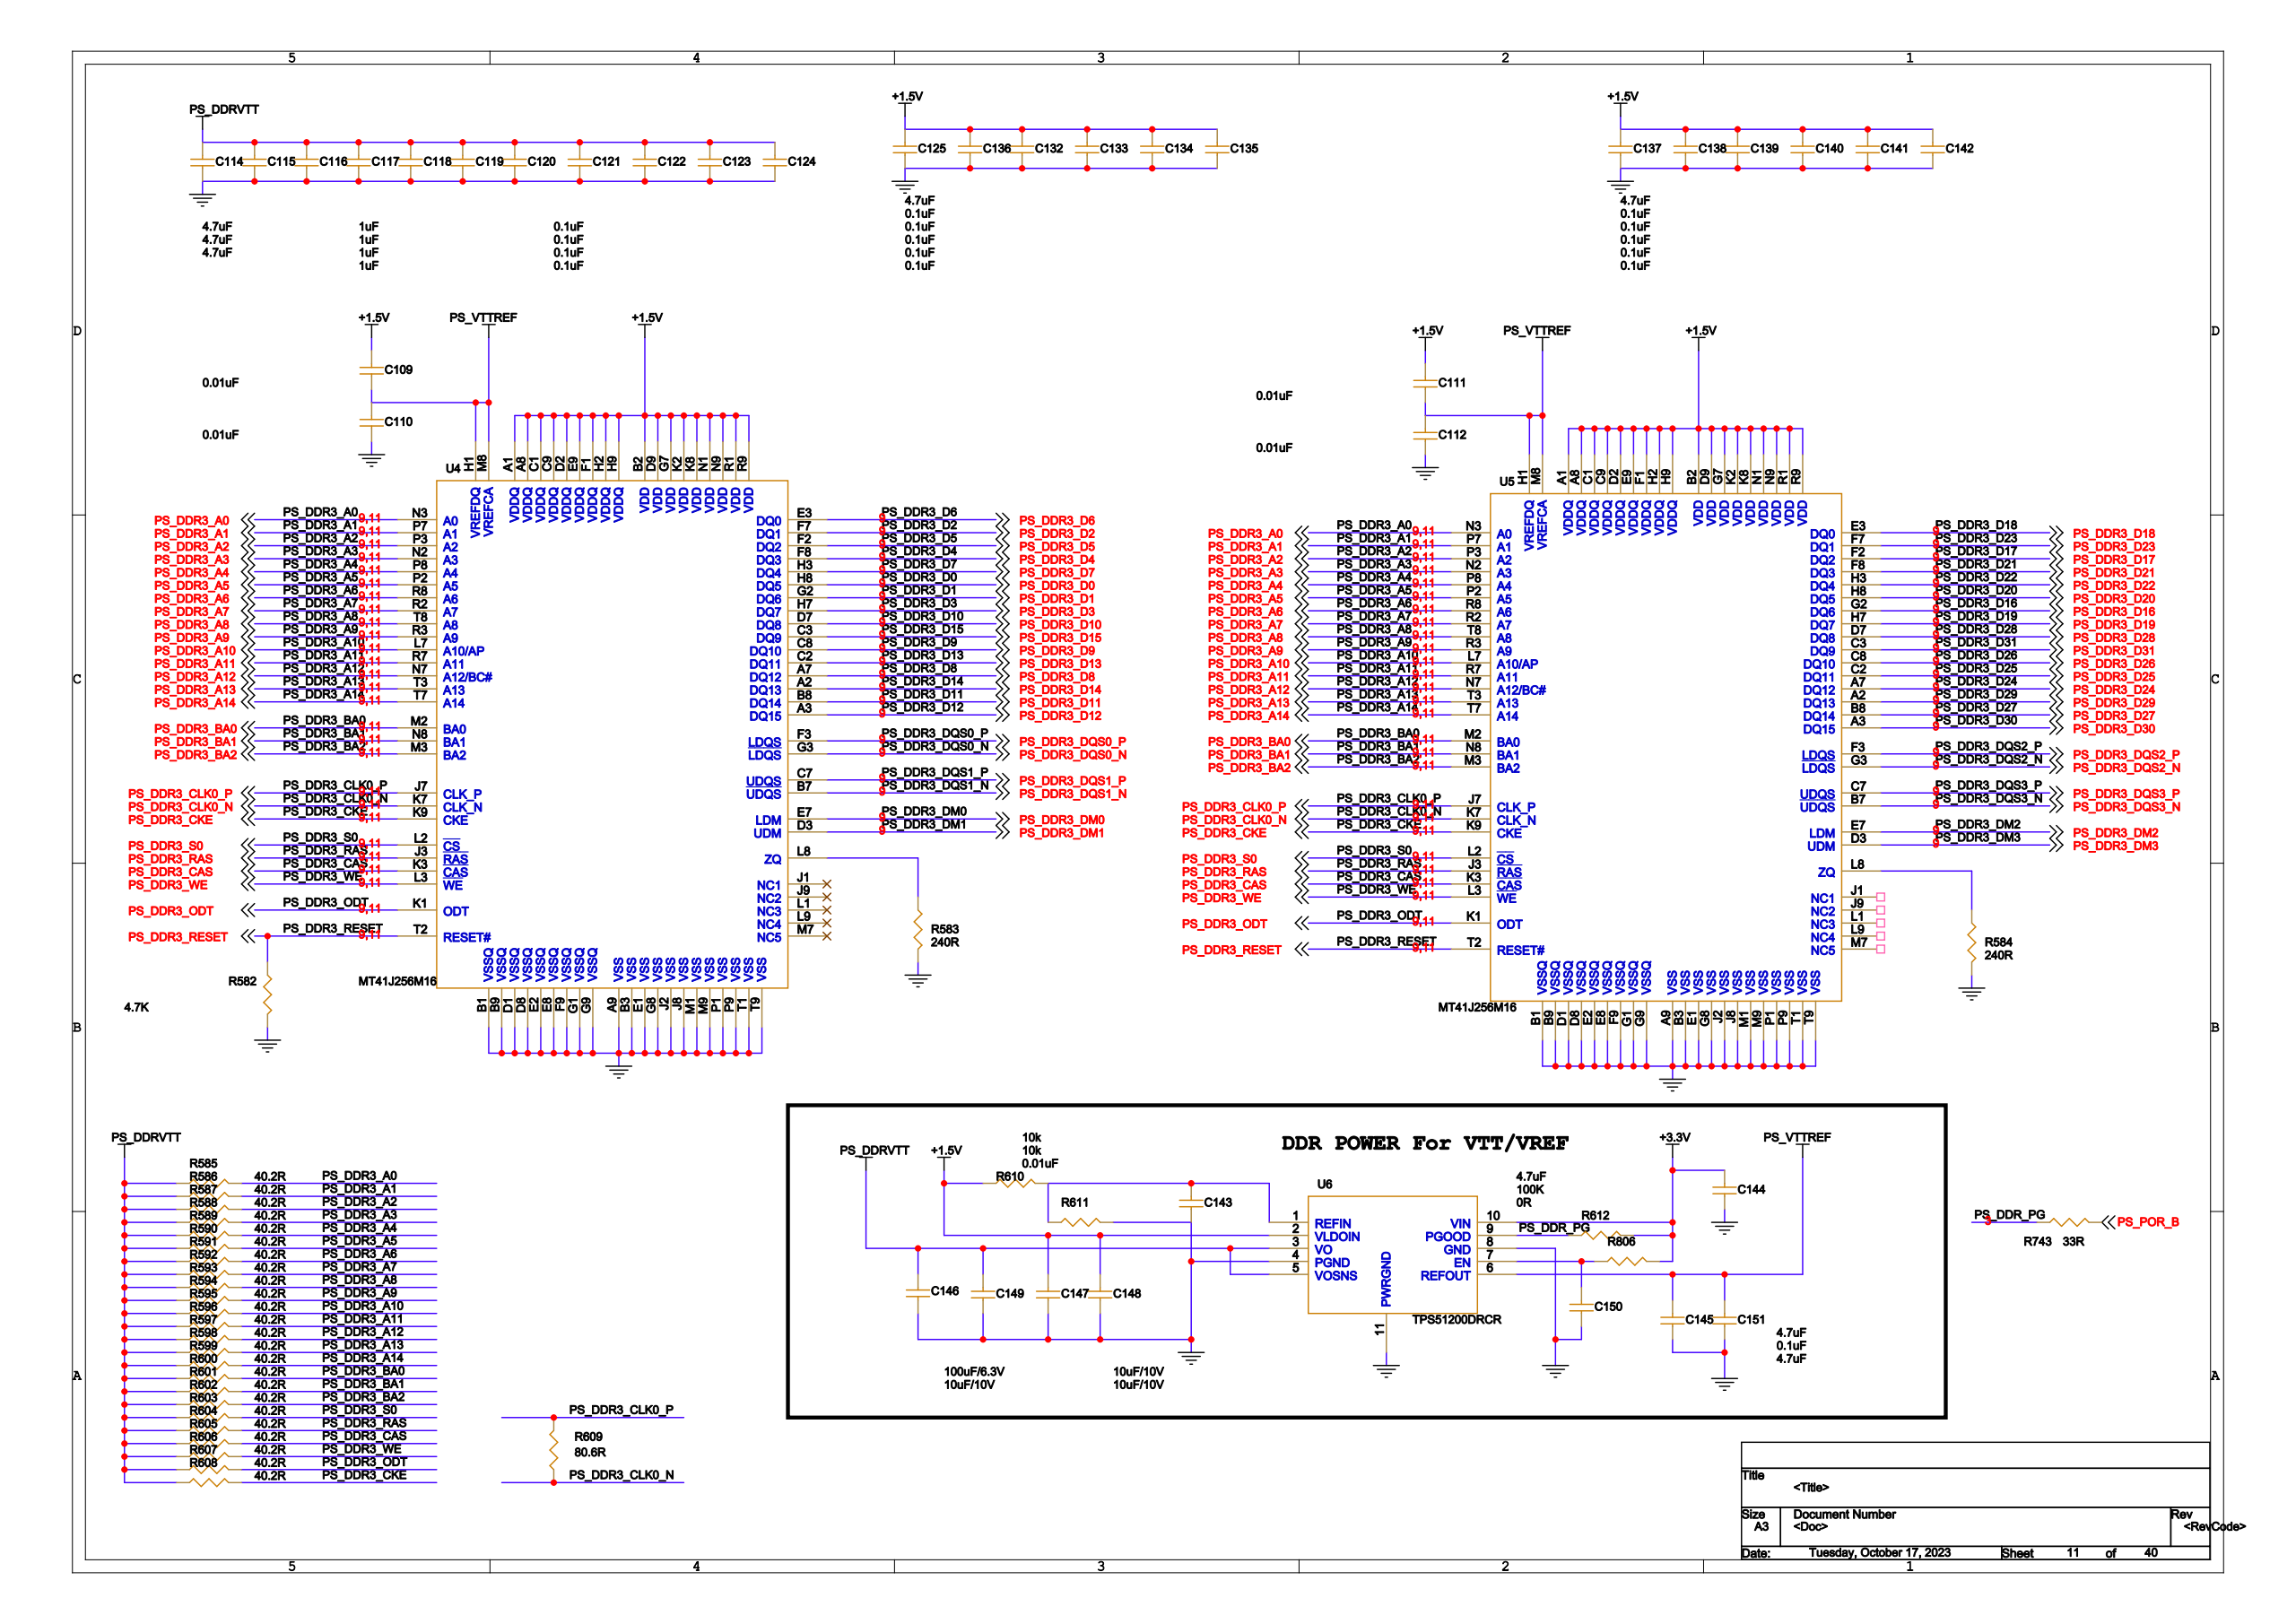Circuit board | Cadence Allegro | 1793 parts | 1223 nets | one sheet of the schematic
Parts on this sheet (reference | value | footprint):
C109 | 0.01uF | C0402
C110 | 0.01uF | C0402
C111 | 0.01uF | C0402
C112 | 0.01uF | C0402
C114 | 4.7uF | C0402
C115 | 4.7uF | C0402
C116 | 4.7uF | C0402
C117 | 1uF | C0402
C118 | 1uF | C0402
C119 | 1uF | C0402
C120 | 1uF | C0402
C121 | 0.1uF | C0402
C122 | 0.1uF | C0402
C123 | 0.1uF | C0402
C124 | 0.1uF | C0402
C125 | 4.7uF | C0402
C132 | 0.1uF | C0402
C133 | 0.1uF | C0402
C134 | 0.1uF | C0402
C135 | 0.1uF | C0402
C136 | 0.1uF | C0402
C137 | 4.7uF | C0402
C138 | 0.1uF | C0402
C139 | 0.1uF | C0402
C140 | 0.1uF | C0402
C141 | 0.1uF | C0402
C142 | 0.1uF | C0402
C143 | 0.01uF | C0402
C144 | 4.7uF | C0402
C145 | 0.1uF | C0402
C146 | 100uF/6.3V | 1206
C147 | 10uF/10V | C0402
C148 | 10uF/10V | C0402
C149 | 10uF/10V | C0402
C150 | 4.7uF | C0402
C151 | 4.7uF | C0402
R582 | 4.7K | R0402
R583 | 240R | R0402
R584 | 240R | R0402
R585 | 40.2R | R0402
R586 | 40.2R | R0402
R587 | 40.2R | R0402
R588 | 40.2R | R0402
R589 | 40.2R | R0402
R590 | 40.2R | R0402
R591 | 40.2R | R0402
R592 | 40.2R | R0402
R593 | 40.2R | R0402
R594 | 40.2R | R0402
R595 | 40.2R | R0402
R596 | 40.2R | R0402
R597 | 40.2R | R0402
R598 | 40.2R | R0402
R599 | 40.2R | R0402
R600 | 40.2R | R0402
R601 | 40.2R | R0402
R602 | 40.2R | R0402
R603 | 40.2R | R0402
R604 | 40.2R | R0402
R605 | 40.2R | R0402
R606 | 40.2R | R0402
R607 | 40.2R | R0402
R608 | 40.2R | R0402
R609 | 80.6R | R0402
R610 | 10k | R0402
R611 | 10k | R0402
R612 | 100K | R0402
R743 | 33R | R0402
R806 | 0R | R0402
U4 | MT41J256M16 | FBGA-96
U5 | MT41J256M16 | FBGA-96
U6 | TPS51200DRCR | TPS51200DRCR
Nets of these parts (net: part-pin ...):
GND: C110-1 C112-1 C114-1 C115-1 C116-1 C117-1 C118-1 C119-1 C120-1 C121-1 C122-1 C123-1 C124-1 C125-1 C132-1 C133-1 C134-1 C135-1 C136-1 C137-1 C138-1 C139-1 C140-1 C141-1 C142-1 C143-1 C144-1 C145-1 C146-2 C147-1 C148-1 C149-1 C150-1 C151-1 R582-1 R583-1 R584-1 R611-1 U6-4 U6-8 U6-11 U4-A9 U4-B1 U4-B3 U4-B9 U4-D1 U4-D8 U4-E1 U4-E2 U4-E8 U4-F9 U4-G1 U4-G8 U4-G9 U4-J2 U4-J8 U4-M1 U4-M9 U4-P1 U4-P9 U4-T1 U4-T9 U5-A9 U5-B1 U5-B3 U5-B9 U5-D1 U5-D8 U5-E1 U5-E2 U5-E8 U5-F9 U5-G1 U5-G8 U5-G9 U5-J2 U5-J8 U5-M1 U5-M9 U5-P1 U5-P9 U5-T1 U5-T9
+1.5V: C109-2 C111-2 C125-2 C132-2 C133-2 C134-2 C135-2 C136-2 C137-2 C138-2 C139-2 C140-2 C141-2 C142-2 C147-2 C148-2 R610-2 U6-2 U4-A1 U4-A8 U4-B2 U4-C1 U4-C9 U4-D2 U4-D9 U4-E9 U4-F1 U4-G7 U4-H2 U4-H9 U4-K2 U4-K8 U4-N1 U4-N9 U4-R1 U4-R9 U5-A1 U5-A8 U5-B2 U5-C1 U5-C9 U5-D2 U5-D9 U5-E9 U5-F1 U5-G7 U5-H2 U5-H9 U5-K2 U5-K8 U5-N1 U5-N9 U5-R1 U5-R9
+3.3V: C144-2 R612-1 R806-1 U6-10
PS_DDRVTT: C114-2 C115-2 C116-2 C117-2 C118-2 C119-2 C120-2 C121-2 C122-2 C123-2 C124-2 C146-1 C149-2 R585-2 R586-2 R587-2 R588-2 R589-2 R590-2 R591-2 R592-2 R593-2 R594-2 R595-2 R596-2 R597-2 R598-2 R599-2 R600-2 R601-2 R602-2 R603-2 R604-2 R605-2 R606-2 R607-2 R608-2 U6-3 U6-5
N146410: C150-2 R806-2 U6-7
PS_VTTREF: C109-1 C110-2 C111-1 C112-2 C145-2 C151-2 U6-6 U4-H1 U4-M8 U5-H1 U5-M8
PS_DDR3_RESET: R582-2 U4-T2 U5-T2
PS_POR_B: R743-1
PS_DDR_PG: R612-2 R743-2 U6-9
PS_DDR3_A0: R585-1 U4-N3 U5-N3
PS_DDR3_A1: R586-1 U4-P7 U5-P7
PS_DDR3_A2: R587-1 U4-P3 U5-P3
PS_DDR3_A3: R588-1 U4-N2 U5-N2
PS_DDR3_A4: R589-1 U4-P8 U5-P8
PS_DDR3_A5: R590-1 U4-P2 U5-P2
PS_DDR3_A6: R591-1 U4-R8 U5-R8
PS_DDR3_A7: R592-1 U4-R2 U5-R2
PS_DDR3_A8: R593-1 U4-T8 U5-T8
PS_DDR3_A9: R594-1 U4-R3 U5-R3
PS_DDR3_A10: R595-1 U4-L7 U5-L7
PS_DDR3_A11: R596-1 U4-R7 U5-R7
PS_DDR3_A12: R597-1 U4-N7 U5-N7
PS_DDR3_A13: R598-1 U4-T3 U5-T3
PS_DDR3_A14: R599-1 U4-T7 U5-T7
PS_DDR3_BA0: R600-1 U4-M2 U5-M2
PS_DDR3_BA1: R601-1 U4-N8 U5-N8
PS_DDR3_BA2: R602-1 U4-M3 U5-M3
PS_DDR3_S0: R603-1 U4-L2 U5-L2
PS_DDR3_RAS: R604-1 U4-J3 U5-J3
PS_DDR3_CAS: R605-1 U4-K3 U5-K3
PS_DDR3_WE: R606-1 U4-L3 U5-L3
PS_DDR3_ODT: R607-1 U4-K1 U5-K1
PS_DDR3_CKE: R608-1 U4-K9 U5-K9
PS_DDR3_CLK0_P: R609-1 U4-J7 U5-J7
PS_DDR3_CLK0_N: R609-2 U4-K7 U5-K7
N124929: R583-2 U4-L8
N128988: R584-2 U5-L8
N143001: C143-2 R610-1 R611-2 U6-1
PS_DDR3_DM0: U4-E7
PS_DDR3_DM1: U4-D3
PS_DDR3_DM2: U5-E7
PS_DDR3_DM3: U5-D3
PS_DDR3_D0: U4-H8
PS_DDR3_D10: U4-D7
PS_DDR3_D11: U4-B8
PS_DDR3_D12: U4-A3
PS_DDR3_D13: U4-C2
PS_DDR3_D14: U4-A2
PS_DDR3_D15: U4-C3
PS_DDR3_D16: U5-G2
PS_DDR3_D17: U5-F2
PS_DDR3_D18: U5-E3
PS_DDR3_D19: U5-H7
PS_DDR3_D1: U4-G2
PS_DDR3_D20: U5-H8
PS_DDR3_D21: U5-F8
PS_DDR3_D22: U5-H3
PS_DDR3_D23: U5-F7
PS_DDR3_D24: U5-A7
PS_DDR3_D25: U5-C2
PS_DDR3_D26: U5-C8
PS_DDR3_D27: U5-B8
PS_DDR3_D28: U5-D7
PS_DDR3_D29: U5-A2
PS_DDR3_D2: U4-F7
PS_DDR3_D30: U5-A3
PS_DDR3_D31: U5-C3
PS_DDR3_D3: U4-H7
PS_DDR3_D4: U4-F8
PS_DDR3_D5: U4-F2
PS_DDR3_D6: U4-E3
PS_DDR3_D7: U4-H3
PS_DDR3_D8: U4-A7
PS_DDR3_D9: U4-C8
PS_DDR3_DQS0_N: U4-G3
PS_DDR3_DQS1_N: U4-B7
PS_DDR3_DQS2_N: U5-G3
PS_DDR3_DQS3_N: U5-B7
PS_DDR3_DQS0_P: U4-F3
PS_DDR3_DQS1_P: U4-C7
PS_DDR3_DQS2_P: U5-F3
PS_DDR3_DQS3_P: U5-C7